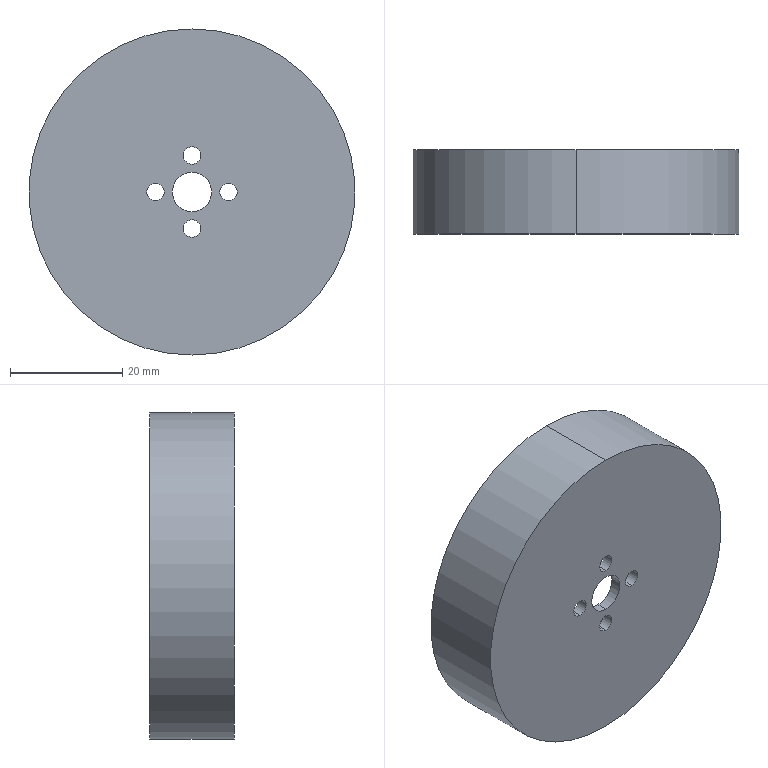Part | SolidWorks | features BaseBody 1 | 1 solid | 17 faces | box 58 x 15 x 58 mm | volume 17889 mm3 | cylinder 14 | plane 3 | commonest cylinder face diameters 3.1 x8 7 x2 46 x2 58 x2
STEP:
#1=CARTESIAN_POINT('',(0.,15.,-29.));
#2=VERTEX_POINT('',#1);
#3=CARTESIAN_POINT('',(0.,15.,29.));
#4=VERTEX_POINT('',#3);
#5=CARTESIAN_POINT('',(0.,15.,0.));
#6=DIRECTION('',(0.,-1.,0.));
#7=DIRECTION('',(0.,0.,-1.));
#8=AXIS2_PLACEMENT_3D('',#5,#6,#7);
#9=CIRCLE('',#8,29.);
#10=EDGE_CURVE('',#2,#4,#9,.T.);
#11=ORIENTED_EDGE('',*,*,#10,.T.);
#12=CARTESIAN_POINT('',(0.,0.,29.));
#13=VERTEX_POINT('',#12);
#14=CARTESIAN_POINT('',(0.,2.,29.));
#15=DIRECTION('',(0.,-1.,0.));
#16=VECTOR('',#15,1000.);
#17=LINE('',#14,#16);
#18=EDGE_CURVE('',#4,#13,#17,.T.);
#19=ORIENTED_EDGE('',*,*,#18,.T.);
#20=CARTESIAN_POINT('',(0.,0.,-29.));
#21=VERTEX_POINT('',#20);
#22=CARTESIAN_POINT('',(0.,0.,0.));
#23=DIRECTION('',(0.,1.,0.));
#24=DIRECTION('',(0.,0.,-1.));
#25=AXIS2_PLACEMENT_3D('',#22,#23,#24);
#26=CIRCLE('',#25,29.);
#27=EDGE_CURVE('',#13,#21,#26,.T.);
#28=ORIENTED_EDGE('',*,*,#27,.T.);
#29=CARTESIAN_POINT('',(0.,2.,-29.));
#30=DIRECTION('',(0.,-1.,0.));
#31=VECTOR('',#30,1000.);
#32=LINE('',#29,#31);
#33=EDGE_CURVE('',#2,#21,#32,.T.);
#34=ORIENTED_EDGE('',*,*,#33,.F.);
#35=EDGE_LOOP('',(#11,#19,#28,#34));
#36=FACE_OUTER_BOUND('',#35,.T.);
#37=CARTESIAN_POINT('',(0.,2.,0.));
#38=DIRECTION('',(0.,-1.,0.));
#39=DIRECTION('',(0.,0.,-1.));
#40=AXIS2_PLACEMENT_3D('',#37,#38,#39);
#41=CYLINDRICAL_SURFACE('',#40,29.);
#42=ADVANCED_FACE('',(#36),#41,.T.);
#43=CARTESIAN_POINT('',(0.,0.,3.5));
#44=VERTEX_POINT('',#43);
#45=CARTESIAN_POINT('',(0.,0.,-3.5));
#46=VERTEX_POINT('',#45);
#47=CARTESIAN_POINT('',(0.,0.,0.));
#48=DIRECTION('',(0.,-1.,0.));
#49=DIRECTION('',(0.,0.,1.));
#50=AXIS2_PLACEMENT_3D('',#47,#48,#49);
#51=CIRCLE('',#50,3.5);
#52=EDGE_CURVE('',#44,#46,#51,.T.);
#53=ORIENTED_EDGE('',*,*,#52,.T.);
#54=CARTESIAN_POINT('',(0.,2.,-3.5));
#55=VERTEX_POINT('',#54);
#56=CARTESIAN_POINT('',(0.,0.,-3.5));
#57=DIRECTION('',(0.,1.,0.));
#58=VECTOR('',#57,1000.);
#59=LINE('',#56,#58);
#60=EDGE_CURVE('',#46,#55,#59,.T.);
#61=ORIENTED_EDGE('',*,*,#60,.T.);
#62=CARTESIAN_POINT('',(0.,2.,3.5));
#63=VERTEX_POINT('',#62);
#64=CARTESIAN_POINT('',(0.,2.,0.));
#65=DIRECTION('',(0.,-1.,0.));
#66=DIRECTION('',(0.,0.,1.));
#67=AXIS2_PLACEMENT_3D('',#64,#65,#66);
#68=CIRCLE('',#67,3.5);
#69=EDGE_CURVE('',#63,#55,#68,.T.);
#70=ORIENTED_EDGE('',*,*,#69,.F.);
#71=CARTESIAN_POINT('',(0.,0.,3.5));
#72=DIRECTION('',(0.,1.,0.));
#73=VECTOR('',#72,1000.);
#74=LINE('',#71,#73);
#75=EDGE_CURVE('',#44,#63,#74,.T.);
#76=ORIENTED_EDGE('',*,*,#75,.F.);
#77=EDGE_LOOP('',(#53,#61,#70,#76));
#78=FACE_OUTER_BOUND('',#77,.T.);
#79=CARTESIAN_POINT('',(0.,0.,0.));
#80=DIRECTION('',(0.,1.,0.));
#81=DIRECTION('',(0.,0.,1.));
#82=AXIS2_PLACEMENT_3D('',#79,#80,#81);
#83=CYLINDRICAL_SURFACE('',#82,3.5);
#84=ADVANCED_FACE('',(#78),#83,.F.);
#85=CARTESIAN_POINT('',(-6.5,2.,1.55));
#86=VERTEX_POINT('',#85);
#87=CARTESIAN_POINT('',(-6.5,2.,-1.55));
#88=VERTEX_POINT('',#87);
#89=CARTESIAN_POINT('',(-6.5,2.,0.));
#90=DIRECTION('',(0.,-1.,0.));
#91=DIRECTION('',(0.,0.,-1.));
#92=AXIS2_PLACEMENT_3D('',#89,#90,#91);
#93=CIRCLE('',#92,1.55);
#94=EDGE_CURVE('',#86,#88,#93,.T.);
#95=ORIENTED_EDGE('',*,*,#94,.F.);
#96=CARTESIAN_POINT('',(-6.5,0.,1.55));
#97=VERTEX_POINT('',#96);
#98=CARTESIAN_POINT('',(-6.5,15.,1.55));
#99=DIRECTION('',(0.,-1.,0.));
#100=VECTOR('',#99,1000.);
#101=LINE('',#98,#100);
#102=EDGE_CURVE('',#86,#97,#101,.T.);
#103=ORIENTED_EDGE('',*,*,#102,.T.);
#104=CARTESIAN_POINT('',(-6.5,0.,-1.55));
#105=VERTEX_POINT('',#104);
#106=CARTESIAN_POINT('',(-6.5,0.,0.));
#107=DIRECTION('',(0.,-1.,0.));
#108=DIRECTION('',(0.,0.,-1.));
#109=AXIS2_PLACEMENT_3D('',#106,#107,#108);
#110=CIRCLE('',#109,1.55);
#111=EDGE_CURVE('',#97,#105,#110,.T.);
#112=ORIENTED_EDGE('',*,*,#111,.T.);
#113=CARTESIAN_POINT('',(-6.5,15.,-1.55));
#114=DIRECTION('',(0.,-1.,0.));
#115=VECTOR('',#114,1000.);
#116=LINE('',#113,#115);
#117=EDGE_CURVE('',#88,#105,#116,.T.);
#118=ORIENTED_EDGE('',*,*,#117,.F.);
#119=EDGE_LOOP('',(#95,#103,#112,#118));
#120=FACE_OUTER_BOUND('',#119,.T.);
#121=CARTESIAN_POINT('',(-6.5,15.,0.));
#122=DIRECTION('',(0.,-1.,0.));
#123=DIRECTION('',(0.,0.,-1.));
#124=AXIS2_PLACEMENT_3D('',#121,#122,#123);
#125=CYLINDRICAL_SURFACE('',#124,1.55);
#126=ADVANCED_FACE('',(#120),#125,.F.);
#127=CARTESIAN_POINT('',(6.5,2.,1.55));
#128=VERTEX_POINT('',#127);
#129=CARTESIAN_POINT('',(6.5,2.,-1.55));
#130=VERTEX_POINT('',#129);
#131=CARTESIAN_POINT('',(6.5,2.,0.));
#132=DIRECTION('',(0.,-1.,0.));
#133=DIRECTION('',(0.,0.,-1.));
#134=AXIS2_PLACEMENT_3D('',#131,#132,#133);
#135=CIRCLE('',#134,1.55);
#136=EDGE_CURVE('',#128,#130,#135,.T.);
#137=ORIENTED_EDGE('',*,*,#136,.F.);
#138=CARTESIAN_POINT('',(6.5,0.,1.55));
#139=VERTEX_POINT('',#138);
#140=CARTESIAN_POINT('',(6.5,15.,1.55));
#141=DIRECTION('',(0.,-1.,0.));
#142=VECTOR('',#141,1000.);
#143=LINE('',#140,#142);
#144=EDGE_CURVE('',#128,#139,#143,.T.);
#145=ORIENTED_EDGE('',*,*,#144,.T.);
#146=CARTESIAN_POINT('',(6.5,0.,-1.55));
#147=VERTEX_POINT('',#146);
#148=CARTESIAN_POINT('',(6.5,0.,0.));
#149=DIRECTION('',(0.,-1.,0.));
#150=DIRECTION('',(0.,0.,-1.));
#151=AXIS2_PLACEMENT_3D('',#148,#149,#150);
#152=CIRCLE('',#151,1.55);
#153=EDGE_CURVE('',#139,#147,#152,.T.);
#154=ORIENTED_EDGE('',*,*,#153,.T.);
#155=CARTESIAN_POINT('',(6.5,15.,-1.55));
#156=DIRECTION('',(0.,-1.,0.));
#157=VECTOR('',#156,1000.);
#158=LINE('',#155,#157);
#159=EDGE_CURVE('',#130,#147,#158,.T.);
#160=ORIENTED_EDGE('',*,*,#159,.F.);
#161=EDGE_LOOP('',(#137,#145,#154,#160));
#162=FACE_OUTER_BOUND('',#161,.T.);
#163=CARTESIAN_POINT('',(6.5,15.,0.));
#164=DIRECTION('',(0.,-1.,0.));
#165=DIRECTION('',(0.,0.,-1.));
#166=AXIS2_PLACEMENT_3D('',#163,#164,#165);
#167=CYLINDRICAL_SURFACE('',#166,1.55);
#168=ADVANCED_FACE('',(#162),#167,.F.);
#169=CARTESIAN_POINT('',(0.,2.,-4.95));
#170=VERTEX_POINT('',#169);
#171=CARTESIAN_POINT('',(0.,2.,-8.05));
#172=VERTEX_POINT('',#171);
#173=CARTESIAN_POINT('',(0.,2.,-6.5));
#174=DIRECTION('',(0.,-1.,0.));
#175=DIRECTION('',(0.,0.,-1.));
#176=AXIS2_PLACEMENT_3D('',#173,#174,#175);
#177=CIRCLE('',#176,1.55);
#178=EDGE_CURVE('',#170,#172,#177,.T.);
#179=ORIENTED_EDGE('',*,*,#178,.F.);
#180=CARTESIAN_POINT('',(0.,0.,-4.95));
#181=VERTEX_POINT('',#180);
#182=CARTESIAN_POINT('',(0.,15.,-4.95));
#183=DIRECTION('',(0.,-1.,0.));
#184=VECTOR('',#183,1000.);
#185=LINE('',#182,#184);
#186=EDGE_CURVE('',#170,#181,#185,.T.);
#187=ORIENTED_EDGE('',*,*,#186,.T.);
#188=CARTESIAN_POINT('',(0.,0.,-8.05));
#189=VERTEX_POINT('',#188);
#190=CARTESIAN_POINT('',(0.,0.,-6.5));
#191=DIRECTION('',(0.,-1.,0.));
#192=DIRECTION('',(0.,0.,-1.));
#193=AXIS2_PLACEMENT_3D('',#190,#191,#192);
#194=CIRCLE('',#193,1.55);
#195=EDGE_CURVE('',#181,#189,#194,.T.);
#196=ORIENTED_EDGE('',*,*,#195,.T.);
#197=CARTESIAN_POINT('',(0.,15.,-8.05));
#198=DIRECTION('',(0.,-1.,0.));
#199=VECTOR('',#198,1000.);
#200=LINE('',#197,#199);
#201=EDGE_CURVE('',#172,#189,#200,.T.);
#202=ORIENTED_EDGE('',*,*,#201,.F.);
#203=EDGE_LOOP('',(#179,#187,#196,#202));
#204=FACE_OUTER_BOUND('',#203,.T.);
#205=CARTESIAN_POINT('',(0.,15.,-6.5));
#206=DIRECTION('',(0.,-1.,0.));
#207=DIRECTION('',(0.,0.,-1.));
#208=AXIS2_PLACEMENT_3D('',#205,#206,#207);
#209=CYLINDRICAL_SURFACE('',#208,1.55);
#210=ADVANCED_FACE('',(#204),#209,.F.);
#211=CARTESIAN_POINT('',(0.,2.,8.05));
#212=VERTEX_POINT('',#211);
#213=CARTESIAN_POINT('',(0.,2.,4.95));
#214=VERTEX_POINT('',#213);
#215=CARTESIAN_POINT('',(0.,2.,6.5));
#216=DIRECTION('',(0.,-1.,0.));
#217=DIRECTION('',(0.,0.,-1.));
#218=AXIS2_PLACEMENT_3D('',#215,#216,#217);
#219=CIRCLE('',#218,1.55);
#220=EDGE_CURVE('',#212,#214,#219,.T.);
#221=ORIENTED_EDGE('',*,*,#220,.F.);
#222=CARTESIAN_POINT('',(0.,0.,8.05));
#223=VERTEX_POINT('',#222);
#224=CARTESIAN_POINT('',(0.,15.,8.05));
#225=DIRECTION('',(0.,-1.,0.));
#226=VECTOR('',#225,1000.);
#227=LINE('',#224,#226);
#228=EDGE_CURVE('',#212,#223,#227,.T.);
#229=ORIENTED_EDGE('',*,*,#228,.T.);
#230=CARTESIAN_POINT('',(0.,0.,4.95));
#231=VERTEX_POINT('',#230);
#232=CARTESIAN_POINT('',(0.,0.,6.5));
#233=DIRECTION('',(0.,-1.,0.));
#234=DIRECTION('',(0.,0.,-1.));
#235=AXIS2_PLACEMENT_3D('',#232,#233,#234);
#236=CIRCLE('',#235,1.55);
#237=EDGE_CURVE('',#223,#231,#236,.T.);
#238=ORIENTED_EDGE('',*,*,#237,.T.);
#239=CARTESIAN_POINT('',(0.,15.,4.95));
#240=DIRECTION('',(0.,-1.,0.));
#241=VECTOR('',#240,1000.);
#242=LINE('',#239,#241);
#243=EDGE_CURVE('',#214,#231,#242,.T.);
#244=ORIENTED_EDGE('',*,*,#243,.F.);
#245=EDGE_LOOP('',(#221,#229,#238,#244));
#246=FACE_OUTER_BOUND('',#245,.T.);
#247=CARTESIAN_POINT('',(0.,15.,6.5));
#248=DIRECTION('',(0.,-1.,0.));
#249=DIRECTION('',(0.,0.,-1.));
#250=AXIS2_PLACEMENT_3D('',#247,#248,#249);
#251=CYLINDRICAL_SURFACE('',#250,1.55);
#252=ADVANCED_FACE('',(#246),#251,.F.);
#253=CARTESIAN_POINT('',(0.,15.,23.));
#254=VERTEX_POINT('',#253);
#255=CARTESIAN_POINT('',(0.,15.,-23.));
#256=VERTEX_POINT('',#255);
#257=CARTESIAN_POINT('',(0.,15.,0.));
#258=DIRECTION('',(0.,-1.,0.));
#259=DIRECTION('',(0.,0.,-1.));
#260=AXIS2_PLACEMENT_3D('',#257,#258,#259);
#261=CIRCLE('',#260,23.);
#262=EDGE_CURVE('',#254,#256,#261,.T.);
#263=ORIENTED_EDGE('',*,*,#262,.F.);
#264=CARTESIAN_POINT('',(0.,2.,23.));
#265=VERTEX_POINT('',#264);
#266=CARTESIAN_POINT('',(0.,15.,23.));
#267=DIRECTION('',(0.,-1.,0.));
#268=VECTOR('',#267,1000.);
#269=LINE('',#266,#268);
#270=EDGE_CURVE('',#254,#265,#269,.T.);
#271=ORIENTED_EDGE('',*,*,#270,.T.);
#272=CARTESIAN_POINT('',(0.,2.,-23.));
#273=VERTEX_POINT('',#272);
#274=CARTESIAN_POINT('',(0.,2.,0.));
#275=DIRECTION('',(0.,1.,0.));
#276=DIRECTION('',(0.,0.,-1.));
#277=AXIS2_PLACEMENT_3D('',#274,#275,#276);
#278=CIRCLE('',#277,23.);
#279=EDGE_CURVE('',#273,#265,#278,.T.);
#280=ORIENTED_EDGE('',*,*,#279,.F.);
#281=CARTESIAN_POINT('',(0.,15.,-23.));
#282=DIRECTION('',(0.,-1.,0.));
#283=VECTOR('',#282,1000.);
#284=LINE('',#281,#283);
#285=EDGE_CURVE('',#256,#273,#284,.T.);
#286=ORIENTED_EDGE('',*,*,#285,.F.);
#287=EDGE_LOOP('',(#263,#271,#280,#286));
#288=FACE_OUTER_BOUND('',#287,.T.);
#289=CARTESIAN_POINT('',(0.,15.,0.));
#290=DIRECTION('',(0.,-1.,0.));
#291=DIRECTION('',(0.,0.,-1.));
#292=AXIS2_PLACEMENT_3D('',#289,#290,#291);
#293=CYLINDRICAL_SURFACE('',#292,23.);
#294=ADVANCED_FACE('',(#288),#293,.F.);
#295=CARTESIAN_POINT('',(0.,0.,0.));
#296=DIRECTION('',(0.,1.,0.));
#297=DIRECTION('',(0.,0.,-1.));
#298=AXIS2_PLACEMENT_3D('',#295,#296,#297);
#299=CIRCLE('',#298,29.);
#300=EDGE_CURVE('',#21,#13,#299,.T.);
#301=ORIENTED_EDGE('',*,*,#300,.F.);
#302=ORIENTED_EDGE('',*,*,#27,.F.);
#303=EDGE_LOOP('',(#301,#302));
#304=FACE_OUTER_BOUND('',#303,.T.);
#305=ORIENTED_EDGE('',*,*,#52,.F.);
#306=CARTESIAN_POINT('',(0.,0.,0.));
#307=DIRECTION('',(0.,-1.,0.));
#308=DIRECTION('',(0.,0.,1.));
#309=AXIS2_PLACEMENT_3D('',#306,#307,#308);
#310=CIRCLE('',#309,3.5);
#311=EDGE_CURVE('',#46,#44,#310,.T.);
#312=ORIENTED_EDGE('',*,*,#311,.F.);
#313=EDGE_LOOP('',(#305,#312));
#314=FACE_BOUND('',#313,.T.);
#315=CARTESIAN_POINT('',(-6.5,0.,0.));
#316=DIRECTION('',(0.,-1.,0.));
#317=DIRECTION('',(0.,0.,-1.));
#318=AXIS2_PLACEMENT_3D('',#315,#316,#317);
#319=CIRCLE('',#318,1.55);
#320=EDGE_CURVE('',#105,#97,#319,.T.);
#321=ORIENTED_EDGE('',*,*,#320,.F.);
#322=ORIENTED_EDGE('',*,*,#111,.F.);
#323=EDGE_LOOP('',(#321,#322));
#324=FACE_BOUND('',#323,.T.);
#325=CARTESIAN_POINT('',(6.5,0.,0.));
#326=DIRECTION('',(0.,-1.,0.));
#327=DIRECTION('',(0.,0.,-1.));
#328=AXIS2_PLACEMENT_3D('',#325,#326,#327);
#329=CIRCLE('',#328,1.55);
#330=EDGE_CURVE('',#147,#139,#329,.T.);
#331=ORIENTED_EDGE('',*,*,#330,.F.);
#332=ORIENTED_EDGE('',*,*,#153,.F.);
#333=EDGE_LOOP('',(#331,#332));
#334=FACE_BOUND('',#333,.T.);
#335=CARTESIAN_POINT('',(0.,0.,-6.5));
#336=DIRECTION('',(0.,-1.,0.));
#337=DIRECTION('',(0.,0.,-1.));
#338=AXIS2_PLACEMENT_3D('',#335,#336,#337);
#339=CIRCLE('',#338,1.55);
#340=EDGE_CURVE('',#189,#181,#339,.T.);
#341=ORIENTED_EDGE('',*,*,#340,.F.);
#342=ORIENTED_EDGE('',*,*,#195,.F.);
#343=EDGE_LOOP('',(#341,#342));
#344=FACE_BOUND('',#343,.T.);
#345=CARTESIAN_POINT('',(0.,0.,6.5));
#346=DIRECTION('',(0.,-1.,0.));
#347=DIRECTION('',(0.,0.,-1.));
#348=AXIS2_PLACEMENT_3D('',#345,#346,#347);
#349=CIRCLE('',#348,1.55);
#350=EDGE_CURVE('',#231,#223,#349,.T.);
#351=ORIENTED_EDGE('',*,*,#350,.F.);
#352=ORIENTED_EDGE('',*,*,#237,.F.);
#353=EDGE_LOOP('',(#351,#352));
#354=FACE_BOUND('',#353,.T.);
#355=CARTESIAN_POINT('',(0.,0.,0.));
#356=DIRECTION('',(0.,1.,0.));
#357=DIRECTION('',(0.,0.,1.));
#358=AXIS2_PLACEMENT_3D('',#355,#356,#357);
#359=PLANE('',#358);
#360=ADVANCED_FACE('',(#304,#314,#324,#334,#344,#354),#359,.F.);
#361=ORIENTED_EDGE('',*,*,#18,.F.);
#362=CARTESIAN_POINT('',(0.,15.,0.));
#363=DIRECTION('',(0.,-1.,0.));
#364=DIRECTION('',(0.,0.,-1.));
#365=AXIS2_PLACEMENT_3D('',#362,#363,#364);
#366=CIRCLE('',#365,29.);
#367=EDGE_CURVE('',#4,#2,#366,.T.);
#368=ORIENTED_EDGE('',*,*,#367,.T.);
#369=ORIENTED_EDGE('',*,*,#33,.T.);
#370=ORIENTED_EDGE('',*,*,#300,.T.);
#371=EDGE_LOOP('',(#361,#368,#369,#370));
#372=FACE_OUTER_BOUND('',#371,.T.);
#373=CARTESIAN_POINT('',(0.,2.,0.));
#374=DIRECTION('',(0.,-1.,0.));
#375=DIRECTION('',(0.,0.,-1.));
#376=AXIS2_PLACEMENT_3D('',#373,#374,#375);
#377=CYLINDRICAL_SURFACE('',#376,29.);
#378=ADVANCED_FACE('',(#372),#377,.T.);
#379=ORIENTED_EDGE('',*,*,#60,.F.);
#380=ORIENTED_EDGE('',*,*,#311,.T.);
#381=ORIENTED_EDGE('',*,*,#75,.T.);
#382=CARTESIAN_POINT('',(0.,2.,0.));
#383=DIRECTION('',(0.,-1.,0.));
#384=DIRECTION('',(0.,0.,1.));
#385=AXIS2_PLACEMENT_3D('',#382,#383,#384);
#386=CIRCLE('',#385,3.5);
#387=EDGE_CURVE('',#55,#63,#386,.T.);
#388=ORIENTED_EDGE('',*,*,#387,.F.);
#389=EDGE_LOOP('',(#379,#380,#381,#388));
#390=FACE_OUTER_BOUND('',#389,.T.);
#391=CARTESIAN_POINT('',(0.,0.,0.));
#392=DIRECTION('',(0.,1.,0.));
#393=DIRECTION('',(0.,0.,1.));
#394=AXIS2_PLACEMENT_3D('',#391,#392,#393);
#395=CYLINDRICAL_SURFACE('',#394,3.5);
#396=ADVANCED_FACE('',(#390),#395,.F.);
#397=ORIENTED_EDGE('',*,*,#102,.F.);
#398=CARTESIAN_POINT('',(-6.5,2.,0.));
#399=DIRECTION('',(0.,-1.,0.));
#400=DIRECTION('',(0.,0.,-1.));
#401=AXIS2_PLACEMENT_3D('',#398,#399,#400);
#402=CIRCLE('',#401,1.55);
#403=EDGE_CURVE('',#88,#86,#402,.T.);
#404=ORIENTED_EDGE('',*,*,#403,.F.);
#405=ORIENTED_EDGE('',*,*,#117,.T.);
#406=ORIENTED_EDGE('',*,*,#320,.T.);
#407=EDGE_LOOP('',(#397,#404,#405,#406));
#408=FACE_OUTER_BOUND('',#407,.T.);
#409=CARTESIAN_POINT('',(-6.5,15.,0.));
#410=DIRECTION('',(0.,-1.,0.));
#411=DIRECTION('',(0.,0.,-1.));
#412=AXIS2_PLACEMENT_3D('',#409,#410,#411);
#413=CYLINDRICAL_SURFACE('',#412,1.55);
#414=ADVANCED_FACE('',(#408),#413,.F.);
#415=ORIENTED_EDGE('',*,*,#144,.F.);
#416=CARTESIAN_POINT('',(6.5,2.,0.));
#417=DIRECTION('',(0.,-1.,0.));
#418=DIRECTION('',(0.,0.,-1.));
#419=AXIS2_PLACEMENT_3D('',#416,#417,#418);
#420=CIRCLE('',#419,1.55);
#421=EDGE_CURVE('',#130,#128,#420,.T.);
#422=ORIENTED_EDGE('',*,*,#421,.F.);
#423=ORIENTED_EDGE('',*,*,#159,.T.);
#424=ORIENTED_EDGE('',*,*,#330,.T.);
#425=EDGE_LOOP('',(#415,#422,#423,#424));
#426=FACE_OUTER_BOUND('',#425,.T.);
#427=CARTESIAN_POINT('',(6.5,15.,0.));
#428=DIRECTION('',(0.,-1.,0.));
#429=DIRECTION('',(0.,0.,-1.));
#430=AXIS2_PLACEMENT_3D('',#427,#428,#429);
#431=CYLINDRICAL_SURFACE('',#430,1.55);
#432=ADVANCED_FACE('',(#426),#431,.F.);
#433=ORIENTED_EDGE('',*,*,#186,.F.);
#434=CARTESIAN_POINT('',(0.,2.,-6.5));
#435=DIRECTION('',(0.,-1.,0.));
#436=DIRECTION('',(0.,0.,-1.));
#437=AXIS2_PLACEMENT_3D('',#434,#435,#436);
#438=CIRCLE('',#437,1.55);
#439=EDGE_CURVE('',#172,#170,#438,.T.);
#440=ORIENTED_EDGE('',*,*,#439,.F.);
#441=ORIENTED_EDGE('',*,*,#201,.T.);
#442=ORIENTED_EDGE('',*,*,#340,.T.);
#443=EDGE_LOOP('',(#433,#440,#441,#442));
#444=FACE_OUTER_BOUND('',#443,.T.);
#445=CARTESIAN_POINT('',(0.,15.,-6.5));
#446=DIRECTION('',(0.,-1.,0.));
#447=DIRECTION('',(0.,0.,-1.));
#448=AXIS2_PLACEMENT_3D('',#445,#446,#447);
#449=CYLINDRICAL_SURFACE('',#448,1.55);
#450=ADVANCED_FACE('',(#444),#449,.F.);
#451=ORIENTED_EDGE('',*,*,#228,.F.);
#452=CARTESIAN_POINT('',(0.,2.,6.5));
#453=DIRECTION('',(0.,-1.,0.));
#454=DIRECTION('',(0.,0.,-1.));
#455=AXIS2_PLACEMENT_3D('',#452,#453,#454);
#456=CIRCLE('',#455,1.55);
#457=EDGE_CURVE('',#214,#212,#456,.T.);
#458=ORIENTED_EDGE('',*,*,#457,.F.);
#459=ORIENTED_EDGE('',*,*,#243,.T.);
#460=ORIENTED_EDGE('',*,*,#350,.T.);
#461=EDGE_LOOP('',(#451,#458,#459,#460));
#462=FACE_OUTER_BOUND('',#461,.T.);
#463=CARTESIAN_POINT('',(0.,15.,6.5));
#464=DIRECTION('',(0.,-1.,0.));
#465=DIRECTION('',(0.,0.,-1.));
#466=AXIS2_PLACEMENT_3D('',#463,#464,#465);
#467=CYLINDRICAL_SURFACE('',#466,1.55);
#468=ADVANCED_FACE('',(#462),#467,.F.);
#469=CARTESIAN_POINT('',(0.,15.,0.));
#470=DIRECTION('',(0.,-1.,0.));
#471=DIRECTION('',(0.,0.,-1.));
#472=AXIS2_PLACEMENT_3D('',#469,#470,#471);
#473=CIRCLE('',#472,23.);
#474=EDGE_CURVE('',#256,#254,#473,.T.);
#475=ORIENTED_EDGE('',*,*,#474,.T.);
#476=ORIENTED_EDGE('',*,*,#262,.T.);
#477=EDGE_LOOP('',(#475,#476));
#478=FACE_BOUND('',#477,.T.);
#479=ORIENTED_EDGE('',*,*,#10,.F.);
#480=ORIENTED_EDGE('',*,*,#367,.F.);
#481=EDGE_LOOP('',(#479,#480));
#482=FACE_OUTER_BOUND('',#481,.T.);
#483=CARTESIAN_POINT('',(0.,15.,0.));
#484=DIRECTION('',(0.,1.,0.));
#485=DIRECTION('',(0.,0.,1.));
#486=AXIS2_PLACEMENT_3D('',#483,#484,#485);
#487=PLANE('',#486);
#488=ADVANCED_FACE('',(#478,#482),#487,.T.);
#489=ORIENTED_EDGE('',*,*,#279,.T.);
#490=CARTESIAN_POINT('',(0.,2.,0.));
#491=DIRECTION('',(0.,1.,0.));
#492=DIRECTION('',(0.,0.,-1.));
#493=AXIS2_PLACEMENT_3D('',#490,#491,#492);
#494=CIRCLE('',#493,23.);
#495=EDGE_CURVE('',#265,#273,#494,.T.);
#496=ORIENTED_EDGE('',*,*,#495,.T.);
#497=EDGE_LOOP('',(#489,#496));
#498=FACE_OUTER_BOUND('',#497,.T.);
#499=ORIENTED_EDGE('',*,*,#69,.T.);
#500=ORIENTED_EDGE('',*,*,#387,.T.);
#501=EDGE_LOOP('',(#499,#500));
#502=FACE_BOUND('',#501,.T.);
#503=ORIENTED_EDGE('',*,*,#403,.T.);
#504=ORIENTED_EDGE('',*,*,#94,.T.);
#505=EDGE_LOOP('',(#503,#504));
#506=FACE_BOUND('',#505,.T.);
#507=ORIENTED_EDGE('',*,*,#421,.T.);
#508=ORIENTED_EDGE('',*,*,#136,.T.);
#509=EDGE_LOOP('',(#507,#508));
#510=FACE_BOUND('',#509,.T.);
#511=ORIENTED_EDGE('',*,*,#439,.T.);
#512=ORIENTED_EDGE('',*,*,#178,.T.);
#513=EDGE_LOOP('',(#511,#512));
#514=FACE_BOUND('',#513,.T.);
#515=ORIENTED_EDGE('',*,*,#457,.T.);
#516=ORIENTED_EDGE('',*,*,#220,.T.);
#517=EDGE_LOOP('',(#515,#516));
#518=FACE_BOUND('',#517,.T.);
#519=CARTESIAN_POINT('',(0.,2.,0.));
#520=DIRECTION('',(0.,1.,0.));
#521=DIRECTION('',(0.,0.,1.));
#522=AXIS2_PLACEMENT_3D('',#519,#520,#521);
#523=PLANE('',#522);
#524=ADVANCED_FACE('',(#498,#502,#506,#510,#514,#518),#523,.T.);
#525=ORIENTED_EDGE('',*,*,#270,.F.);
#526=ORIENTED_EDGE('',*,*,#474,.F.);
#527=ORIENTED_EDGE('',*,*,#285,.T.);
#528=ORIENTED_EDGE('',*,*,#495,.F.);
#529=EDGE_LOOP('',(#525,#526,#527,#528));
#530=FACE_OUTER_BOUND('',#529,.T.);
#531=CARTESIAN_POINT('',(0.,15.,0.));
#532=DIRECTION('',(0.,-1.,0.));
#533=DIRECTION('',(0.,0.,-1.));
#534=AXIS2_PLACEMENT_3D('',#531,#532,#533);
#535=CYLINDRICAL_SURFACE('',#534,23.);
#536=ADVANCED_FACE('',(#530),#535,.F.);
#537=CLOSED_SHELL('',(#42,#84,#126,#168,#210,#252,#294,#360,#378,#396,#414,#432,#450,#468,#488,#524,#536));
#538=MANIFOLD_SOLID_BREP('',#537);
#539=CARTESIAN_POINT('',(0.,0.,0.));
#540=DIRECTION('',(0.,0.,1.));
#541=DIRECTION('',(1.,0.,0.));
#542=AXIS2_PLACEMENT_3D('',#539,#540,#541);
#543=(LENGTH_UNIT()NAMED_UNIT(*)SI_UNIT(.MILLI.,.METRE.));
#544=UNCERTAINTY_MEASURE_WITH_UNIT(LENGTH_MEASURE(0.00001),#543,'','');
#545=(NAMED_UNIT(*)PLANE_ANGLE_UNIT()SI_UNIT($,.RADIAN.));
#546=(NAMED_UNIT(*)SI_UNIT($,.STERADIAN.)SOLID_ANGLE_UNIT());
#547=(GEOMETRIC_REPRESENTATION_CONTEXT(3)GLOBAL_UNCERTAINTY_ASSIGNED_CONTEXT((#544))GLOBAL_UNIT_ASSIGNED_CONTEXT((#543,#545,#546))REPRESENTATION_CONTEXT('',''));
#548=ADVANCED_BREP_SHAPE_REPRESENTATION('',(#538,#542),#547);